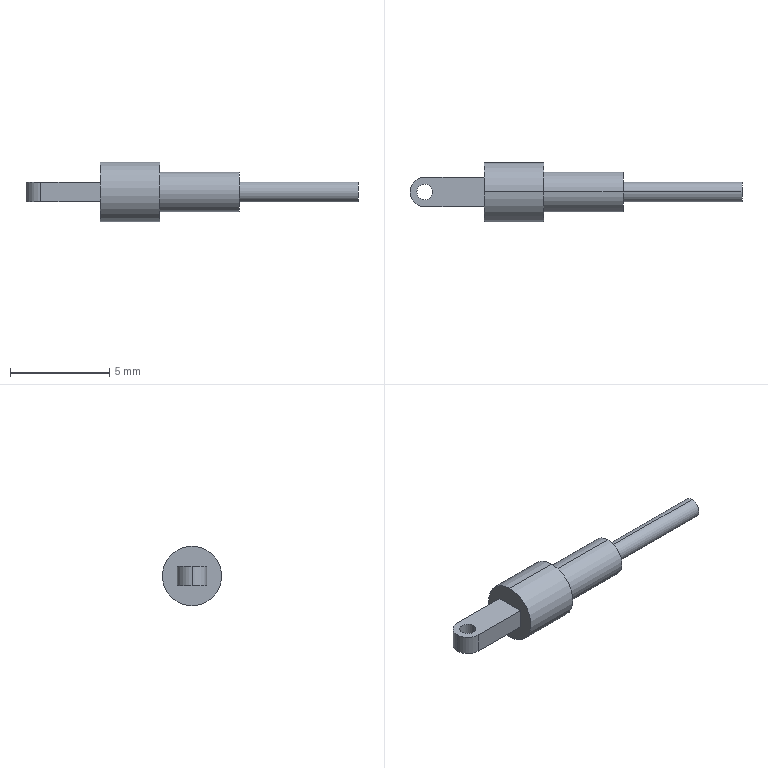Part | SolidWorks | features ICE 2, Revolution 1 | 1 solid | 18 faces | box 16.75 x 3 x 3 mm | volume 43.365 mm3 | cylinder 10 | plane 8 | commonest cylinder face diameters 0.8 x2 1 x2 1.5 x2 2 x2 3 x2
STEP:
#1=CARTESIAN_POINT('',(7.,0.,-0.5));
#2=VERTEX_POINT('',#1);
#3=CARTESIAN_POINT('',(7.,0.,0.5));
#4=VERTEX_POINT('',#3);
#5=CARTESIAN_POINT('',(7.,0.,0.));
#6=DIRECTION('',(1.,0.,0.));
#7=DIRECTION('',(0.,0.,-1.));
#8=AXIS2_PLACEMENT_3D('',#5,#6,#7);
#9=CIRCLE('',#8,0.5);
#10=EDGE_CURVE('',#2,#4,#9,.T.);
#11=ORIENTED_EDGE('',*,*,#10,.T.);
#12=CARTESIAN_POINT('',(13.,0.,0.5));
#13=VERTEX_POINT('',#12);
#14=CARTESIAN_POINT('',(7.,0.,0.5));
#15=DIRECTION('',(1.,0.,0.));
#16=VECTOR('',#15,1000.);
#17=LINE('',#14,#16);
#18=EDGE_CURVE('',#4,#13,#17,.T.);
#19=ORIENTED_EDGE('',*,*,#18,.T.);
#20=CARTESIAN_POINT('',(13.,0.,-0.5));
#21=VERTEX_POINT('',#20);
#22=CARTESIAN_POINT('',(13.,0.,0.));
#23=DIRECTION('',(1.,0.,0.));
#24=DIRECTION('',(0.,0.,-1.));
#25=AXIS2_PLACEMENT_3D('',#22,#23,#24);
#26=CIRCLE('',#25,0.5);
#27=EDGE_CURVE('',#21,#13,#26,.T.);
#28=ORIENTED_EDGE('',*,*,#27,.F.);
#29=CARTESIAN_POINT('',(7.,0.,-0.5));
#30=DIRECTION('',(1.,0.,0.));
#31=VECTOR('',#30,1000.);
#32=LINE('',#29,#31);
#33=EDGE_CURVE('',#2,#21,#32,.T.);
#34=ORIENTED_EDGE('',*,*,#33,.F.);
#35=EDGE_LOOP('',(#11,#19,#28,#34));
#36=FACE_OUTER_BOUND('',#35,.T.);
#37=CARTESIAN_POINT('',(7.,0.,0.));
#38=DIRECTION('',(1.,0.,0.));
#39=DIRECTION('',(0.,0.,-1.));
#40=AXIS2_PLACEMENT_3D('',#37,#38,#39);
#41=CYLINDRICAL_SURFACE('',#40,0.5);
#42=ADVANCED_FACE('',(#36),#41,.T.);
#43=CARTESIAN_POINT('',(-3.4,0.,0.5));
#44=VERTEX_POINT('',#43);
#45=CARTESIAN_POINT('',(-2.6,0.,0.5));
#46=VERTEX_POINT('',#45);
#47=CARTESIAN_POINT('',(-3.,0.,0.5));
#48=DIRECTION('',(0.,0.,1.));
#49=DIRECTION('',(1.,0.,0.));
#50=AXIS2_PLACEMENT_3D('',#47,#48,#49);
#51=CIRCLE('',#50,0.4);
#52=EDGE_CURVE('',#44,#46,#51,.T.);
#53=ORIENTED_EDGE('',*,*,#52,.T.);
#54=CARTESIAN_POINT('',(-2.6,0.,-0.5));
#55=VERTEX_POINT('',#54);
#56=CARTESIAN_POINT('',(-2.6,0.,0.5));
#57=DIRECTION('',(0.,0.,-1.));
#58=VECTOR('',#57,1000.);
#59=LINE('',#56,#58);
#60=EDGE_CURVE('',#46,#55,#59,.T.);
#61=ORIENTED_EDGE('',*,*,#60,.T.);
#62=CARTESIAN_POINT('',(-3.4,0.,-0.5));
#63=VERTEX_POINT('',#62);
#64=CARTESIAN_POINT('',(-3.,0.,-0.5));
#65=DIRECTION('',(0.,0.,1.));
#66=DIRECTION('',(1.,0.,0.));
#67=AXIS2_PLACEMENT_3D('',#64,#65,#66);
#68=CIRCLE('',#67,0.4);
#69=EDGE_CURVE('',#63,#55,#68,.T.);
#70=ORIENTED_EDGE('',*,*,#69,.F.);
#71=CARTESIAN_POINT('',(-3.4,0.,0.5));
#72=DIRECTION('',(0.,0.,-1.));
#73=VECTOR('',#72,1000.);
#74=LINE('',#71,#73);
#75=EDGE_CURVE('',#44,#63,#74,.T.);
#76=ORIENTED_EDGE('',*,*,#75,.F.);
#77=EDGE_LOOP('',(#53,#61,#70,#76));
#78=FACE_OUTER_BOUND('',#77,.T.);
#79=CARTESIAN_POINT('',(-3.,0.,0.5));
#80=DIRECTION('',(0.,0.,-1.));
#81=DIRECTION('',(-1.,0.,0.));
#82=AXIS2_PLACEMENT_3D('',#79,#80,#81);
#83=CYLINDRICAL_SURFACE('',#82,0.4);
#84=ADVANCED_FACE('',(#78),#83,.F.);
#85=CARTESIAN_POINT('',(-3.75,0.,0.5));
#86=VERTEX_POINT('',#85);
#87=CARTESIAN_POINT('',(-3.,-0.75,0.5));
#88=VERTEX_POINT('',#87);
#89=CARTESIAN_POINT('',(-3.,0.,0.5));
#90=DIRECTION('',(0.,0.,1.));
#91=DIRECTION('',(-1.,0.,0.));
#92=AXIS2_PLACEMENT_3D('',#89,#90,#91);
#93=CIRCLE('',#92,0.75);
#94=EDGE_CURVE('',#86,#88,#93,.T.);
#95=ORIENTED_EDGE('',*,*,#94,.F.);
#96=CARTESIAN_POINT('',(-3.75,0.,-0.5));
#97=VERTEX_POINT('',#96);
#98=CARTESIAN_POINT('',(-3.75,0.,0.5));
#99=DIRECTION('',(0.,0.,-1.));
#100=VECTOR('',#99,1000.);
#101=LINE('',#98,#100);
#102=EDGE_CURVE('',#86,#97,#101,.T.);
#103=ORIENTED_EDGE('',*,*,#102,.T.);
#104=CARTESIAN_POINT('',(-3.,-0.75,-0.5));
#105=VERTEX_POINT('',#104);
#106=CARTESIAN_POINT('',(-3.,0.,-0.5));
#107=DIRECTION('',(0.,0.,1.));
#108=DIRECTION('',(-1.,0.,0.));
#109=AXIS2_PLACEMENT_3D('',#106,#107,#108);
#110=CIRCLE('',#109,0.75);
#111=EDGE_CURVE('',#97,#105,#110,.T.);
#112=ORIENTED_EDGE('',*,*,#111,.T.);
#113=CARTESIAN_POINT('',(-3.,-0.75,0.5));
#114=DIRECTION('',(0.,0.,-1.));
#115=VECTOR('',#114,1000.);
#116=LINE('',#113,#115);
#117=EDGE_CURVE('',#88,#105,#116,.T.);
#118=ORIENTED_EDGE('',*,*,#117,.F.);
#119=EDGE_LOOP('',(#95,#103,#112,#118));
#120=FACE_OUTER_BOUND('',#119,.T.);
#121=CARTESIAN_POINT('',(-3.,0.,0.5));
#122=DIRECTION('',(0.,0.,-1.));
#123=DIRECTION('',(-1.,0.,0.));
#124=AXIS2_PLACEMENT_3D('',#121,#122,#123);
#125=CYLINDRICAL_SURFACE('',#124,0.75);
#126=ADVANCED_FACE('',(#120),#125,.T.);
#127=CARTESIAN_POINT('',(3.,0.,1.5));
#128=VERTEX_POINT('',#127);
#129=CARTESIAN_POINT('',(3.,0.,-1.5));
#130=VERTEX_POINT('',#129);
#131=CARTESIAN_POINT('',(3.,0.,0.));
#132=DIRECTION('',(-1.,0.,0.));
#133=DIRECTION('',(0.,0.,1.));
#134=AXIS2_PLACEMENT_3D('',#131,#132,#133);
#135=CIRCLE('',#134,1.5);
#136=EDGE_CURVE('',#128,#130,#135,.T.);
#137=ORIENTED_EDGE('',*,*,#136,.T.);
#138=CARTESIAN_POINT('',(0.,0.,-1.5));
#139=VERTEX_POINT('',#138);
#140=CARTESIAN_POINT('',(0.1244,0.,-1.5));
#141=DIRECTION('',(-1.,0.,0.));
#142=VECTOR('',#141,1000.);
#143=LINE('',#140,#142);
#144=EDGE_CURVE('',#130,#139,#143,.T.);
#145=ORIENTED_EDGE('',*,*,#144,.T.);
#146=CARTESIAN_POINT('',(0.,0.,1.5));
#147=VERTEX_POINT('',#146);
#148=CARTESIAN_POINT('',(0.,0.,0.));
#149=DIRECTION('',(-1.,0.,0.));
#150=DIRECTION('',(0.,0.,1.));
#151=AXIS2_PLACEMENT_3D('',#148,#149,#150);
#152=CIRCLE('',#151,1.5);
#153=EDGE_CURVE('',#147,#139,#152,.T.);
#154=ORIENTED_EDGE('',*,*,#153,.F.);
#155=CARTESIAN_POINT('',(0.1244,0.,1.5));
#156=DIRECTION('',(-1.,0.,0.));
#157=VECTOR('',#156,1000.);
#158=LINE('',#155,#157);
#159=EDGE_CURVE('',#128,#147,#158,.T.);
#160=ORIENTED_EDGE('',*,*,#159,.F.);
#161=EDGE_LOOP('',(#137,#145,#154,#160));
#162=FACE_OUTER_BOUND('',#161,.T.);
#163=CARTESIAN_POINT('',(0.1244,0.,0.));
#164=DIRECTION('',(-1.,0.,0.));
#165=DIRECTION('',(0.,0.,1.));
#166=AXIS2_PLACEMENT_3D('',#163,#164,#165);
#167=CYLINDRICAL_SURFACE('',#166,1.5);
#168=ADVANCED_FACE('',(#162),#167,.T.);
#169=CARTESIAN_POINT('',(7.,0.,-1.));
#170=VERTEX_POINT('',#169);
#171=CARTESIAN_POINT('',(7.,0.,1.));
#172=VERTEX_POINT('',#171);
#173=CARTESIAN_POINT('',(7.,0.,0.));
#174=DIRECTION('',(1.,0.,0.));
#175=DIRECTION('',(0.,0.,-1.));
#176=AXIS2_PLACEMENT_3D('',#173,#174,#175);
#177=CIRCLE('',#176,1.);
#178=EDGE_CURVE('',#170,#172,#177,.T.);
#179=ORIENTED_EDGE('',*,*,#178,.F.);
#180=CARTESIAN_POINT('',(3.,0.,-1.));
#181=VERTEX_POINT('',#180);
#182=CARTESIAN_POINT('',(0.1244,0.,-1.));
#183=DIRECTION('',(-1.,0.,0.));
#184=VECTOR('',#183,1000.);
#185=LINE('',#182,#184);
#186=EDGE_CURVE('',#170,#181,#185,.T.);
#187=ORIENTED_EDGE('',*,*,#186,.T.);
#188=CARTESIAN_POINT('',(3.,0.,1.));
#189=VERTEX_POINT('',#188);
#190=CARTESIAN_POINT('',(3.,0.,0.));
#191=DIRECTION('',(-1.,0.,0.));
#192=DIRECTION('',(0.,0.,1.));
#193=AXIS2_PLACEMENT_3D('',#190,#191,#192);
#194=CIRCLE('',#193,1.);
#195=EDGE_CURVE('',#189,#181,#194,.T.);
#196=ORIENTED_EDGE('',*,*,#195,.F.);
#197=CARTESIAN_POINT('',(0.1244,0.,1.));
#198=DIRECTION('',(-1.,0.,0.));
#199=VECTOR('',#198,1000.);
#200=LINE('',#197,#199);
#201=EDGE_CURVE('',#172,#189,#200,.T.);
#202=ORIENTED_EDGE('',*,*,#201,.F.);
#203=EDGE_LOOP('',(#179,#187,#196,#202));
#204=FACE_OUTER_BOUND('',#203,.T.);
#205=CARTESIAN_POINT('',(0.1244,0.,0.));
#206=DIRECTION('',(-1.,0.,0.));
#207=DIRECTION('',(0.,0.,1.));
#208=AXIS2_PLACEMENT_3D('',#205,#206,#207);
#209=CYLINDRICAL_SURFACE('',#208,1.);
#210=ADVANCED_FACE('',(#204),#209,.T.);
#211=ORIENTED_EDGE('',*,*,#186,.F.);
#212=CARTESIAN_POINT('',(7.,0.,0.));
#213=DIRECTION('',(1.,0.,0.));
#214=DIRECTION('',(0.,0.,-1.));
#215=AXIS2_PLACEMENT_3D('',#212,#213,#214);
#216=CIRCLE('',#215,1.);
#217=EDGE_CURVE('',#172,#170,#216,.T.);
#218=ORIENTED_EDGE('',*,*,#217,.F.);
#219=ORIENTED_EDGE('',*,*,#201,.T.);
#220=CARTESIAN_POINT('',(3.,0.,0.));
#221=DIRECTION('',(-1.,0.,0.));
#222=DIRECTION('',(0.,0.,1.));
#223=AXIS2_PLACEMENT_3D('',#220,#221,#222);
#224=CIRCLE('',#223,1.);
#225=EDGE_CURVE('',#181,#189,#224,.T.);
#226=ORIENTED_EDGE('',*,*,#225,.F.);
#227=EDGE_LOOP('',(#211,#218,#219,#226));
#228=FACE_OUTER_BOUND('',#227,.T.);
#229=CARTESIAN_POINT('',(0.1244,0.,0.));
#230=DIRECTION('',(-1.,0.,0.));
#231=DIRECTION('',(0.,0.,1.));
#232=AXIS2_PLACEMENT_3D('',#229,#230,#231);
#233=CYLINDRICAL_SURFACE('',#232,1.);
#234=ADVANCED_FACE('',(#228),#233,.T.);
#235=CARTESIAN_POINT('',(0.,-0.75,0.5));
#236=VERTEX_POINT('',#235);
#237=CARTESIAN_POINT('',(0.,-0.75,-0.5));
#238=VERTEX_POINT('',#237);
#239=CARTESIAN_POINT('',(0.,-0.75,0.5));
#240=DIRECTION('',(0.,0.,-1.));
#241=VECTOR('',#240,1000.);
#242=LINE('',#239,#241);
#243=EDGE_CURVE('',#236,#238,#242,.T.);
#244=ORIENTED_EDGE('',*,*,#243,.T.);
#245=CARTESIAN_POINT('',(0.,0.75,-0.5));
#246=VERTEX_POINT('',#245);
#247=CARTESIAN_POINT('',(0.,0.75,-0.5));
#248=DIRECTION('',(0.,1.,0.));
#249=VECTOR('',#248,1000.);
#250=LINE('',#247,#249);
#251=EDGE_CURVE('',#238,#246,#250,.T.);
#252=ORIENTED_EDGE('',*,*,#251,.T.);
#253=CARTESIAN_POINT('',(0.,0.75,0.5));
#254=VERTEX_POINT('',#253);
#255=CARTESIAN_POINT('',(0.,0.75,0.5));
#256=DIRECTION('',(0.,0.,-1.));
#257=VECTOR('',#256,1000.);
#258=LINE('',#255,#257);
#259=EDGE_CURVE('',#254,#246,#258,.T.);
#260=ORIENTED_EDGE('',*,*,#259,.F.);
#261=CARTESIAN_POINT('',(0.,0.75,0.5));
#262=DIRECTION('',(0.,1.,0.));
#263=VECTOR('',#262,1000.);
#264=LINE('',#261,#263);
#265=EDGE_CURVE('',#236,#254,#264,.T.);
#266=ORIENTED_EDGE('',*,*,#265,.F.);
#267=EDGE_LOOP('',(#244,#252,#260,#266));
#268=FACE_BOUND('',#267,.T.);
#269=ORIENTED_EDGE('',*,*,#153,.T.);
#270=CARTESIAN_POINT('',(0.,0.,0.));
#271=DIRECTION('',(-1.,0.,0.));
#272=DIRECTION('',(0.,0.,1.));
#273=AXIS2_PLACEMENT_3D('',#270,#271,#272);
#274=CIRCLE('',#273,1.5);
#275=EDGE_CURVE('',#139,#147,#274,.T.);
#276=ORIENTED_EDGE('',*,*,#275,.T.);
#277=EDGE_LOOP('',(#269,#276));
#278=FACE_OUTER_BOUND('',#277,.T.);
#279=CARTESIAN_POINT('',(0.,0.,0.));
#280=DIRECTION('',(1.,0.,0.));
#281=DIRECTION('',(0.,0.,-1.));
#282=AXIS2_PLACEMENT_3D('',#279,#280,#281);
#283=PLANE('',#282);
#284=ADVANCED_FACE('',(#268,#278),#283,.F.);
#285=ORIENTED_EDGE('',*,*,#144,.F.);
#286=CARTESIAN_POINT('',(3.,0.,0.));
#287=DIRECTION('',(-1.,0.,0.));
#288=DIRECTION('',(0.,0.,1.));
#289=AXIS2_PLACEMENT_3D('',#286,#287,#288);
#290=CIRCLE('',#289,1.5);
#291=EDGE_CURVE('',#130,#128,#290,.T.);
#292=ORIENTED_EDGE('',*,*,#291,.T.);
#293=ORIENTED_EDGE('',*,*,#159,.T.);
#294=ORIENTED_EDGE('',*,*,#275,.F.);
#295=EDGE_LOOP('',(#285,#292,#293,#294));
#296=FACE_OUTER_BOUND('',#295,.T.);
#297=CARTESIAN_POINT('',(0.1244,0.,0.));
#298=DIRECTION('',(-1.,0.,0.));
#299=DIRECTION('',(0.,0.,1.));
#300=AXIS2_PLACEMENT_3D('',#297,#298,#299);
#301=CYLINDRICAL_SURFACE('',#300,1.5);
#302=ADVANCED_FACE('',(#296),#301,.T.);
#303=ORIENTED_EDGE('',*,*,#136,.F.);
#304=ORIENTED_EDGE('',*,*,#291,.F.);
#305=EDGE_LOOP('',(#303,#304));
#306=FACE_OUTER_BOUND('',#305,.T.);
#307=ORIENTED_EDGE('',*,*,#195,.T.);
#308=ORIENTED_EDGE('',*,*,#225,.T.);
#309=EDGE_LOOP('',(#307,#308));
#310=FACE_BOUND('',#309,.T.);
#311=CARTESIAN_POINT('',(3.,1.5,0.));
#312=DIRECTION('',(-1.,0.,0.));
#313=DIRECTION('',(0.,0.,1.));
#314=AXIS2_PLACEMENT_3D('',#311,#312,#313);
#315=PLANE('',#314);
#316=ADVANCED_FACE('',(#306,#310),#315,.F.);
#317=CARTESIAN_POINT('',(0.,-0.75,0.5));
#318=DIRECTION('',(1.,0.,0.));
#319=VECTOR('',#318,1000.);
#320=LINE('',#317,#319);
#321=EDGE_CURVE('',#88,#236,#320,.T.);
#322=ORIENTED_EDGE('',*,*,#321,.T.);
#323=ORIENTED_EDGE('',*,*,#265,.T.);
#324=CARTESIAN_POINT('',(-3.,0.75,0.5));
#325=VERTEX_POINT('',#324);
#326=CARTESIAN_POINT('',(0.,0.75,0.5));
#327=DIRECTION('',(-1.,0.,0.));
#328=VECTOR('',#327,1000.);
#329=LINE('',#326,#328);
#330=EDGE_CURVE('',#254,#325,#329,.T.);
#331=ORIENTED_EDGE('',*,*,#330,.T.);
#332=CARTESIAN_POINT('',(-3.,0.,0.5));
#333=DIRECTION('',(0.,0.,1.));
#334=DIRECTION('',(-1.,0.,0.));
#335=AXIS2_PLACEMENT_3D('',#332,#333,#334);
#336=CIRCLE('',#335,0.75);
#337=EDGE_CURVE('',#325,#86,#336,.T.);
#338=ORIENTED_EDGE('',*,*,#337,.T.);
#339=ORIENTED_EDGE('',*,*,#94,.T.);
#340=EDGE_LOOP('',(#322,#323,#331,#338,#339));
#341=FACE_OUTER_BOUND('',#340,.T.);
#342=ORIENTED_EDGE('',*,*,#52,.F.);
#343=CARTESIAN_POINT('',(-3.,0.,0.5));
#344=DIRECTION('',(0.,0.,1.));
#345=DIRECTION('',(1.,0.,0.));
#346=AXIS2_PLACEMENT_3D('',#343,#344,#345);
#347=CIRCLE('',#346,0.4);
#348=EDGE_CURVE('',#46,#44,#347,.T.);
#349=ORIENTED_EDGE('',*,*,#348,.F.);
#350=EDGE_LOOP('',(#342,#349));
#351=FACE_BOUND('',#350,.T.);
#352=CARTESIAN_POINT('',(-3.,0.,0.5));
#353=DIRECTION('',(0.,0.,-1.));
#354=DIRECTION('',(-1.,0.,0.));
#355=AXIS2_PLACEMENT_3D('',#352,#353,#354);
#356=PLANE('',#355);
#357=ADVANCED_FACE('',(#341,#351),#356,.F.);
#358=CARTESIAN_POINT('',(0.,-0.75,-0.5));
#359=DIRECTION('',(1.,0.,0.));
#360=VECTOR('',#359,1000.);
#361=LINE('',#358,#360);
#362=EDGE_CURVE('',#105,#238,#361,.T.);
#363=ORIENTED_EDGE('',*,*,#362,.F.);
#364=ORIENTED_EDGE('',*,*,#111,.F.);
#365=CARTESIAN_POINT('',(-3.,0.75,-0.5));
#366=VERTEX_POINT('',#365);
#367=CARTESIAN_POINT('',(-3.,0.,-0.5));
#368=DIRECTION('',(0.,0.,1.));
#369=DIRECTION('',(-1.,0.,0.));
#370=AXIS2_PLACEMENT_3D('',#367,#368,#369);
#371=CIRCLE('',#370,0.75);
#372=EDGE_CURVE('',#366,#97,#371,.T.);
#373=ORIENTED_EDGE('',*,*,#372,.F.);
#374=CARTESIAN_POINT('',(0.,0.75,-0.5));
#375=DIRECTION('',(-1.,0.,0.));
#376=VECTOR('',#375,1000.);
#377=LINE('',#374,#376);
#378=EDGE_CURVE('',#246,#366,#377,.T.);
#379=ORIENTED_EDGE('',*,*,#378,.F.);
#380=ORIENTED_EDGE('',*,*,#251,.F.);
#381=EDGE_LOOP('',(#363,#364,#373,#379,#380));
#382=FACE_OUTER_BOUND('',#381,.T.);
#383=ORIENTED_EDGE('',*,*,#69,.T.);
#384=CARTESIAN_POINT('',(-3.,0.,-0.5));
#385=DIRECTION('',(0.,0.,1.));
#386=DIRECTION('',(1.,0.,0.));
#387=AXIS2_PLACEMENT_3D('',#384,#385,#386);
#388=CIRCLE('',#387,0.4);
#389=EDGE_CURVE('',#55,#63,#388,.T.);
#390=ORIENTED_EDGE('',*,*,#389,.T.);
#391=EDGE_LOOP('',(#383,#390));
#392=FACE_BOUND('',#391,.T.);
#393=CARTESIAN_POINT('',(-3.,0.,-0.5));
#394=DIRECTION('',(0.,0.,-1.));
#395=DIRECTION('',(-1.,0.,0.));
#396=AXIS2_PLACEMENT_3D('',#393,#394,#395);
#397=PLANE('',#396);
#398=ADVANCED_FACE('',(#382,#392),#397,.T.);
#399=ORIENTED_EDGE('',*,*,#362,.T.);
#400=ORIENTED_EDGE('',*,*,#243,.F.);
#401=ORIENTED_EDGE('',*,*,#321,.F.);
#402=ORIENTED_EDGE('',*,*,#117,.T.);
#403=EDGE_LOOP('',(#399,#400,#401,#402));
#404=FACE_OUTER_BOUND('',#403,.T.);
#405=CARTESIAN_POINT('',(0.,-0.75,0.5));
#406=DIRECTION('',(0.,1.,0.));
#407=DIRECTION('',(-1.,0.,0.));
#408=AXIS2_PLACEMENT_3D('',#405,#406,#407);
#409=PLANE('',#408);
#410=ADVANCED_FACE('',(#404),#409,.F.);
#411=ORIENTED_EDGE('',*,*,#378,.T.);
#412=CARTESIAN_POINT('',(-3.,0.75,0.5));
#413=DIRECTION('',(0.,0.,-1.));
#414=VECTOR('',#413,1000.);
#415=LINE('',#412,#414);
#416=EDGE_CURVE('',#325,#366,#415,.T.);
#417=ORIENTED_EDGE('',*,*,#416,.F.);
#418=ORIENTED_EDGE('',*,*,#330,.F.);
#419=ORIENTED_EDGE('',*,*,#259,.T.);
#420=EDGE_LOOP('',(#411,#417,#418,#419));
#421=FACE_OUTER_BOUND('',#420,.T.);
#422=CARTESIAN_POINT('',(0.,0.75,0.5));
#423=DIRECTION('',(0.,-1.,0.));
#424=DIRECTION('',(1.,0.,0.));
#425=AXIS2_PLACEMENT_3D('',#422,#423,#424);
#426=PLANE('',#425);
#427=ADVANCED_FACE('',(#421),#426,.F.);
#428=ORIENTED_EDGE('',*,*,#102,.F.);
#429=ORIENTED_EDGE('',*,*,#337,.F.);
#430=ORIENTED_EDGE('',*,*,#416,.T.);
#431=ORIENTED_EDGE('',*,*,#372,.T.);
#432=EDGE_LOOP('',(#428,#429,#430,#431));
#433=FACE_OUTER_BOUND('',#432,.T.);
#434=CARTESIAN_POINT('',(-3.,0.,0.5));
#435=DIRECTION('',(0.,0.,-1.));
#436=DIRECTION('',(-1.,0.,0.));
#437=AXIS2_PLACEMENT_3D('',#434,#435,#436);
#438=CYLINDRICAL_SURFACE('',#437,0.75);
#439=ADVANCED_FACE('',(#433),#438,.T.);
#440=ORIENTED_EDGE('',*,*,#60,.F.);
#441=ORIENTED_EDGE('',*,*,#348,.T.);
#442=ORIENTED_EDGE('',*,*,#75,.T.);
#443=ORIENTED_EDGE('',*,*,#389,.F.);
#444=EDGE_LOOP('',(#440,#441,#442,#443));
#445=FACE_OUTER_BOUND('',#444,.T.);
#446=CARTESIAN_POINT('',(-3.,0.,0.5));
#447=DIRECTION('',(0.,0.,-1.));
#448=DIRECTION('',(-1.,0.,0.));
#449=AXIS2_PLACEMENT_3D('',#446,#447,#448);
#450=CYLINDRICAL_SURFACE('',#449,0.4);
#451=ADVANCED_FACE('',(#445),#450,.F.);
#452=ORIENTED_EDGE('',*,*,#10,.F.);
#453=CARTESIAN_POINT('',(7.,0.,0.));
#454=DIRECTION('',(1.,0.,0.));
#455=DIRECTION('',(0.,0.,-1.));
#456=AXIS2_PLACEMENT_3D('',#453,#454,#455);
#457=CIRCLE('',#456,0.5);
#458=EDGE_CURVE('',#4,#2,#457,.T.);
#459=ORIENTED_EDGE('',*,*,#458,.F.);
#460=EDGE_LOOP('',(#452,#459));
#461=FACE_BOUND('',#460,.T.);
#462=ORIENTED_EDGE('',*,*,#217,.T.);
#463=ORIENTED_EDGE('',*,*,#178,.T.);
#464=EDGE_LOOP('',(#462,#463));
#465=FACE_OUTER_BOUND('',#464,.T.);
#466=CARTESIAN_POINT('',(7.,0.,0.));
#467=DIRECTION('',(1.,0.,0.));
#468=DIRECTION('',(0.,0.,-1.));
#469=AXIS2_PLACEMENT_3D('',#466,#467,#468);
#470=PLANE('',#469);
#471=ADVANCED_FACE('',(#461,#465),#470,.T.);
#472=ORIENTED_EDGE('',*,*,#18,.F.);
#473=ORIENTED_EDGE('',*,*,#458,.T.);
#474=ORIENTED_EDGE('',*,*,#33,.T.);
#475=CARTESIAN_POINT('',(13.,0.,0.));
#476=DIRECTION('',(1.,0.,0.));
#477=DIRECTION('',(0.,0.,-1.));
#478=AXIS2_PLACEMENT_3D('',#475,#476,#477);
#479=CIRCLE('',#478,0.5);
#480=EDGE_CURVE('',#13,#21,#479,.T.);
#481=ORIENTED_EDGE('',*,*,#480,.F.);
#482=EDGE_LOOP('',(#472,#473,#474,#481));
#483=FACE_OUTER_BOUND('',#482,.T.);
#484=CARTESIAN_POINT('',(7.,0.,0.));
#485=DIRECTION('',(1.,0.,0.));
#486=DIRECTION('',(0.,0.,-1.));
#487=AXIS2_PLACEMENT_3D('',#484,#485,#486);
#488=CYLINDRICAL_SURFACE('',#487,0.5);
#489=ADVANCED_FACE('',(#483),#488,.T.);
#490=ORIENTED_EDGE('',*,*,#27,.T.);
#491=ORIENTED_EDGE('',*,*,#480,.T.);
#492=EDGE_LOOP('',(#490,#491));
#493=FACE_OUTER_BOUND('',#492,.T.);
#494=CARTESIAN_POINT('',(13.,1.,0.));
#495=DIRECTION('',(-1.,0.,0.));
#496=DIRECTION('',(0.,0.,1.));
#497=AXIS2_PLACEMENT_3D('',#494,#495,#496);
#498=PLANE('',#497);
#499=ADVANCED_FACE('',(#493),#498,.F.);
#500=CLOSED_SHELL('',(#42,#84,#126,#168,#210,#234,#284,#302,#316,#357,#398,#410,#427,#439,#451,#471,#489,#499));
#501=MANIFOLD_SOLID_BREP('',#500);
#502=CARTESIAN_POINT('',(0.,0.,0.));
#503=DIRECTION('',(0.,0.,1.));
#504=DIRECTION('',(1.,0.,0.));
#505=AXIS2_PLACEMENT_3D('',#502,#503,#504);
#506=(LENGTH_UNIT()NAMED_UNIT(*)SI_UNIT(.MILLI.,.METRE.));
#507=UNCERTAINTY_MEASURE_WITH_UNIT(LENGTH_MEASURE(0.00001),#506,'','');
#508=(NAMED_UNIT(*)PLANE_ANGLE_UNIT()SI_UNIT($,.RADIAN.));
#509=(NAMED_UNIT(*)SI_UNIT($,.STERADIAN.)SOLID_ANGLE_UNIT());
#510=(GEOMETRIC_REPRESENTATION_CONTEXT(3)GLOBAL_UNCERTAINTY_ASSIGNED_CONTEXT((#507))GLOBAL_UNIT_ASSIGNED_CONTEXT((#506,#508,#509))REPRESENTATION_CONTEXT('',''));
#511=ADVANCED_BREP_SHAPE_REPRESENTATION('',(#501,#505),#510);